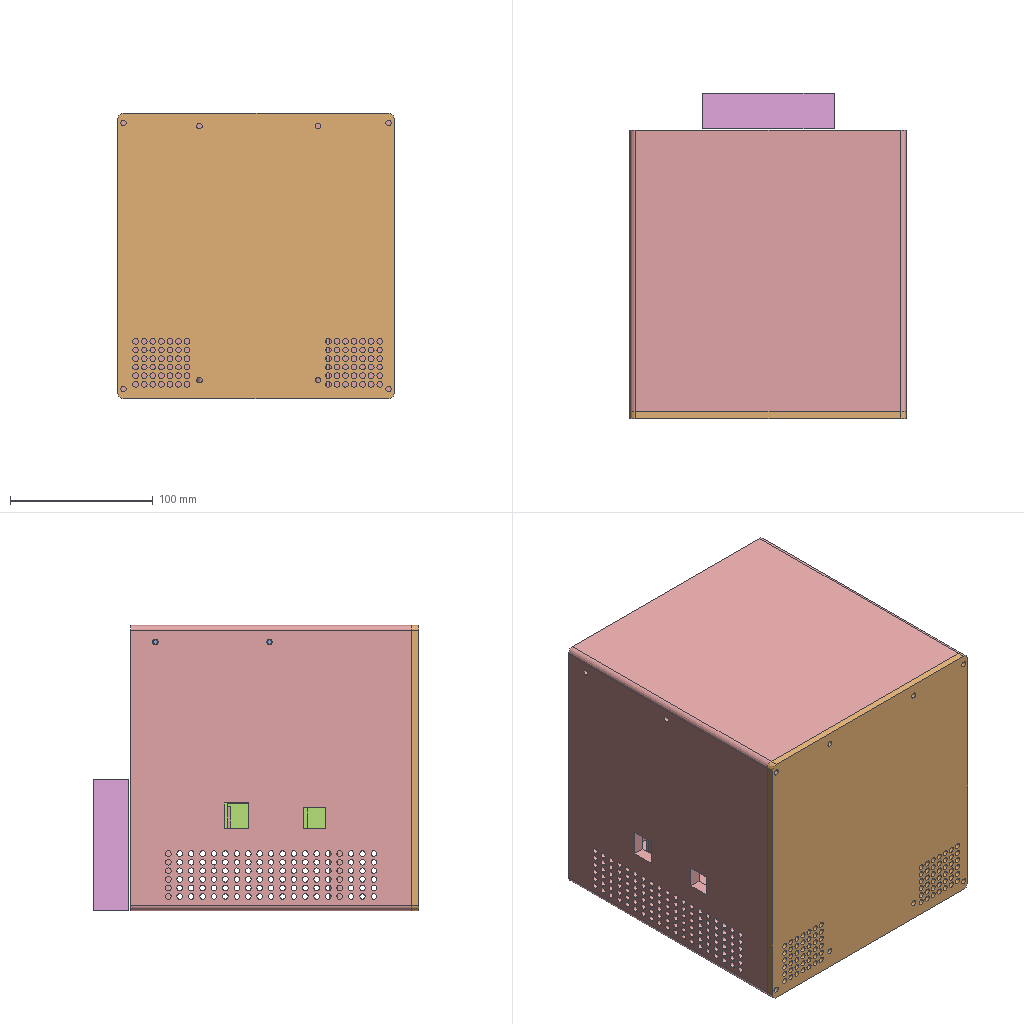Assembly | SolidWorks | 8 different items | 10 placed | box 194 x 228 x 200 mm
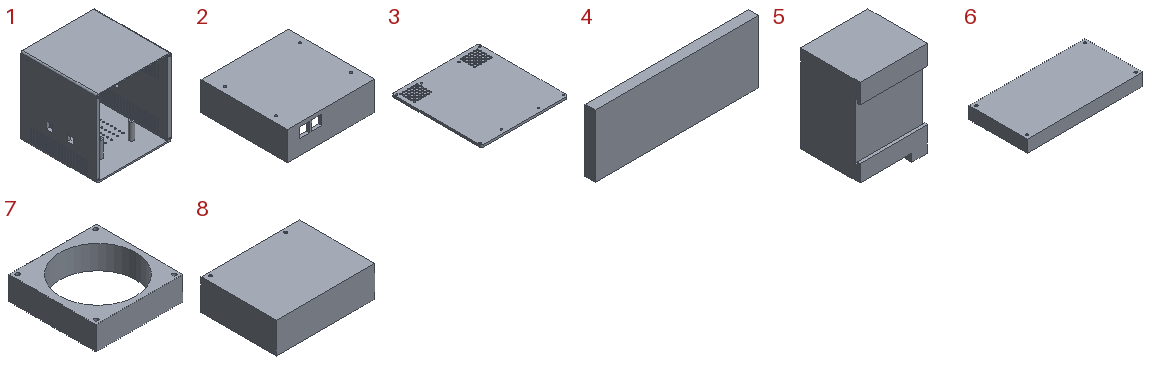Parts list (item | quantity | size | volume | features):
1 | x1 | 193.595 x 197 x 200 mm | 952035 mm3 | features ICE 18, OffsetRefSurface 2, Thicken 2, BossThin 1, Chamfer 1, Extrusion 1, Fillet 1, LPattern 1, MirrorPattern 1, Shell 1
2 | x1 | 140 x 138 x 46 mm | 201014 mm3 | features ICE 9, Extrusion 1, Shell 1
3 | x1 | 193.6 x 200 x 5 mm | 187754 mm3 | features ICE 3, Extrusion 1, Fillet 1, LPattern 1
4 | x1 | 131 x 8 x 50 mm | 51646 mm3 | features Extrusion 1, ICE 1
5 | x3 | 42.7 x 37.7 x 60.3 mm | 84935 mm3 | features Cut 1, Extrusion 1, ICE 1
6 | x1 | 190 x 95 x 20 mm | 28754 mm3 | features ICE 9, Extrusion 1, Shell 1
7 | x1 | 92 x 92 x 25 mm | 84680 mm3 | features ICE 2, Extrusion 1
8 | x1 | 105 x 80.181 x 33 mm | 28220 mm3 | features Extrusion 1, ICE 1, Shell 1
Mates (type | each side: item.copy, entity, surface, feature):
Coincident | 1.1 face plane Boss-Extrude1 | 6.1 face plane Boss-Extrude1
Coincident | 1.1 face plane Shell2 | 6.1 face plane Boss-Extrude1
Parallel | 1.1 face plane Shell2 | 8.1 face plane Boss-Extrude1
Coincident | 1.1 face plane Boss-Extrude1 | 7.1 face plane Boss-Extrude1
Concentric | 1.1 face cylinder Cut-Extrude7 | 8.1 face cylinder Cut-Extrude2 | 2 times
Coincident | 1.1 face plane Thicken1 | 3.1 face plane Boss-Extrude1
Coincident | 1.1 face plane Boss-Extrude1 | 3.1 face plane Boss-Extrude1 | 2 times
Coincident | 5.1 face plane Boss-Extrude1 | 5.2 face plane Boss-Extrude1 | 3 times
Coincident | 5.2 face plane Boss-Extrude1 | 5.3 face plane Boss-Extrude1 | 3 times
DistanceDim | 1.1 face plane Shell2 | 2.1 face plane Boss-Extrude1
Parallel | 1.1 face plane Boss-Extrude1 | 4.1 face plane Boss-Extrude1 | 2 times
DistanceDim | 1.1 face plane Shell2 | 4.1 face plane Boss-Extrude1
DistanceDim | 4.1 face plane Boss-Extrude1 | 1.1 face plane Shell2
Coincident | 1.1 face plane Shell2 | 4.1 face plane Boss-Extrude1